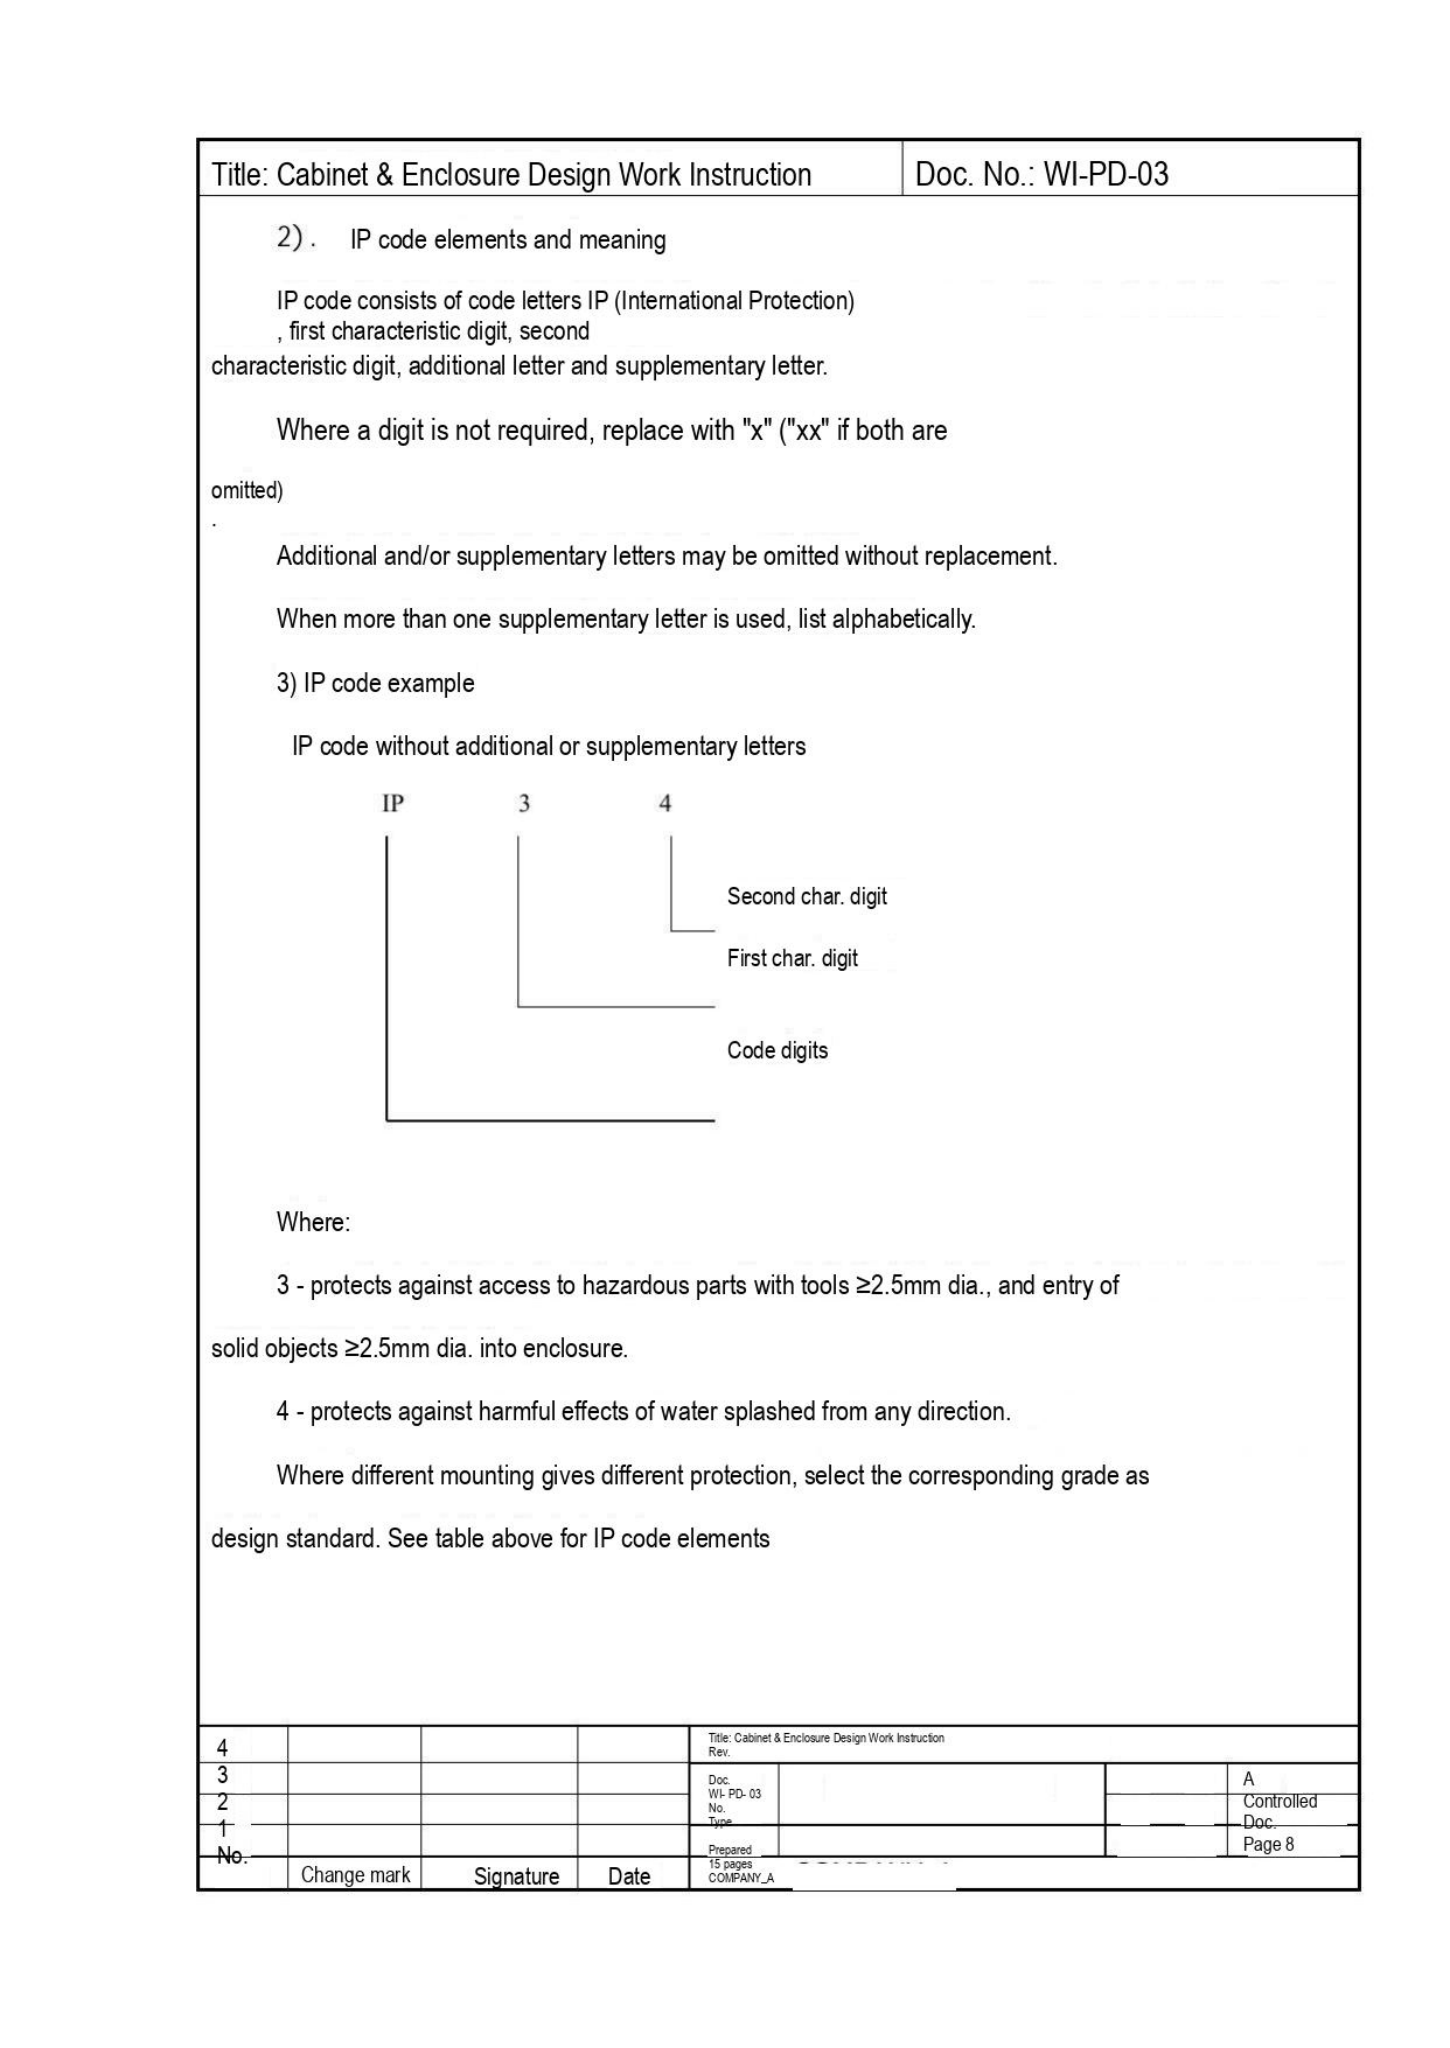| Title: Cabinet & Enclosure Design Work Instruction | Doc. No.: WI-PD-03 |
|---|---|

2）. IP code elements and meaning

IP code consists of code letters IP (International Protection), first characteristic digit, second characteristic digit, additional letter and supplementary letter.

Where a digit is not required, replace with "x" ("xx" if both are omitted).

Additional and/or supplementary letters may be omitted without replacement.

When more than one supplementary letter is used, list alphabetically.

3) IP code example

IP code without additional or supplementary letters

IP 3 4

Second char. digit

First char. digit

Code digits

Where:

3 - protects against access to hazardous parts with tools ≥2.5mm dia., and entry of solid objects ≥2.5mm dia. into enclosure.

4 - protects against harmful effects of water splashed from any direction.

Where different mounting gives different protection, select the corresponding grade as design standard. See table above for IP code elements

| No. | Change mark | Signature | Date |
|---|---|---|---|
| 4 | | | |
| 3 | | | |
| 2 | | | |
| 1 | | | |

Title: Cabinet & Enclosure Design Work Instruction
Rev.
Doc. No. WI- PD- 03
Type
Prepared
15 pages
COMPANY_A
A
Controlled Doc.
Page 8
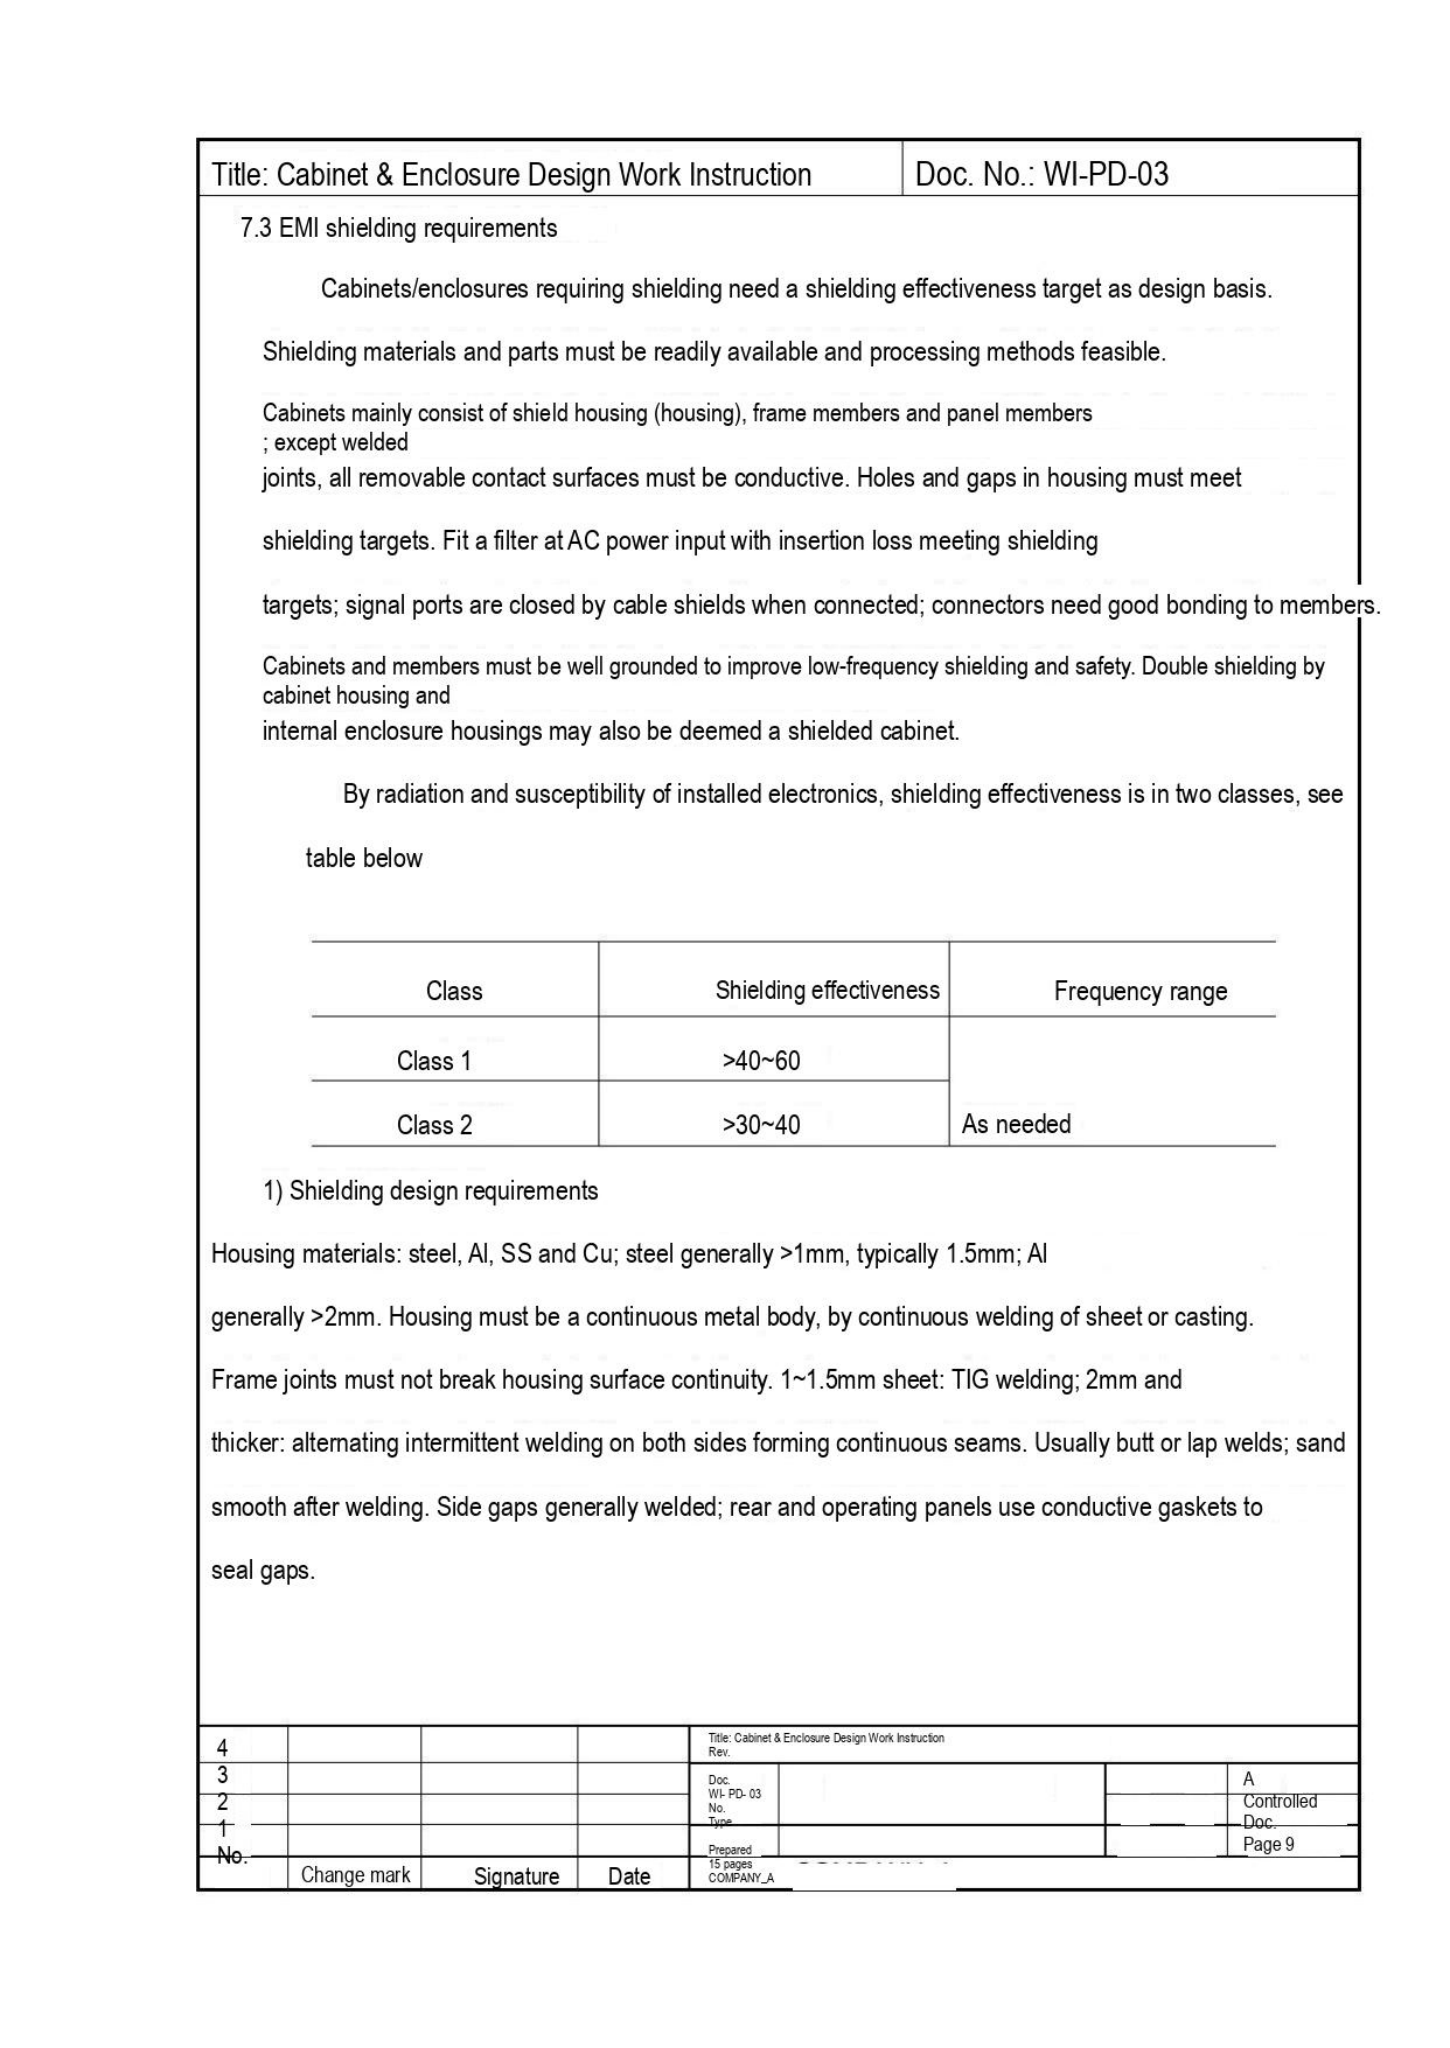Title: Cabinet & Enclosure Design Work Instruction | Doc. No.: WI-PD-03

7.3 EMI shielding requirements

Cabinets/enclosures requiring shielding need a shielding effectiveness target as design basis.

Shielding materials and parts must be readily available and processing methods feasible.

Cabinets mainly consist of shield housing (housing), frame members and panel members ; except welded joints, all removable contact surfaces must be conductive. Holes and gaps in housing must meet shielding targets. Fit a filter at AC power input with insertion loss meeting shielding targets; signal ports are closed by cable shields when connected; connectors need good bonding to members.

Cabinets and members must be well grounded to improve low-frequency shielding and safety. Double shielding by cabinet housing and internal enclosure housings may also be deemed a shielded cabinet.

By radiation and susceptibility of installed electronics, shielding effectiveness is in two classes, see table below

| Class | Shielding effectiveness | Frequency range |
|---|---|---|
| Class 1 | >40~60 | As needed |
| Class 2 | >30~40 | |

1) Shielding design requirements

Housing materials: steel, Al, SS and Cu; steel generally >1mm, typically 1.5mm; Al generally >2mm. Housing must be a continuous metal body, by continuous welding of sheet or casting. Frame joints must not break housing surface continuity. 1~1.5mm sheet: TIG welding; 2mm and thicker: alternating intermittent welding on both sides forming continuous seams. Usually butt or lap welds; sand smooth after welding. Side gaps generally welded; rear and operating panels use conductive gaskets to seal gaps.

| No. | Change mark | Signature | Date |
|---|---|---|---|
| 4 | | | |
| 3 | | | |
| 2 | | | |
| 1 | | | |

Title: Cabinet & Enclosure Design Work Instruction
Rev.
Doc.
WI- PD- 03
No.
Type
Prepared
15 pages
COMPANY_A
A
Controlled
Doc.
Page 9
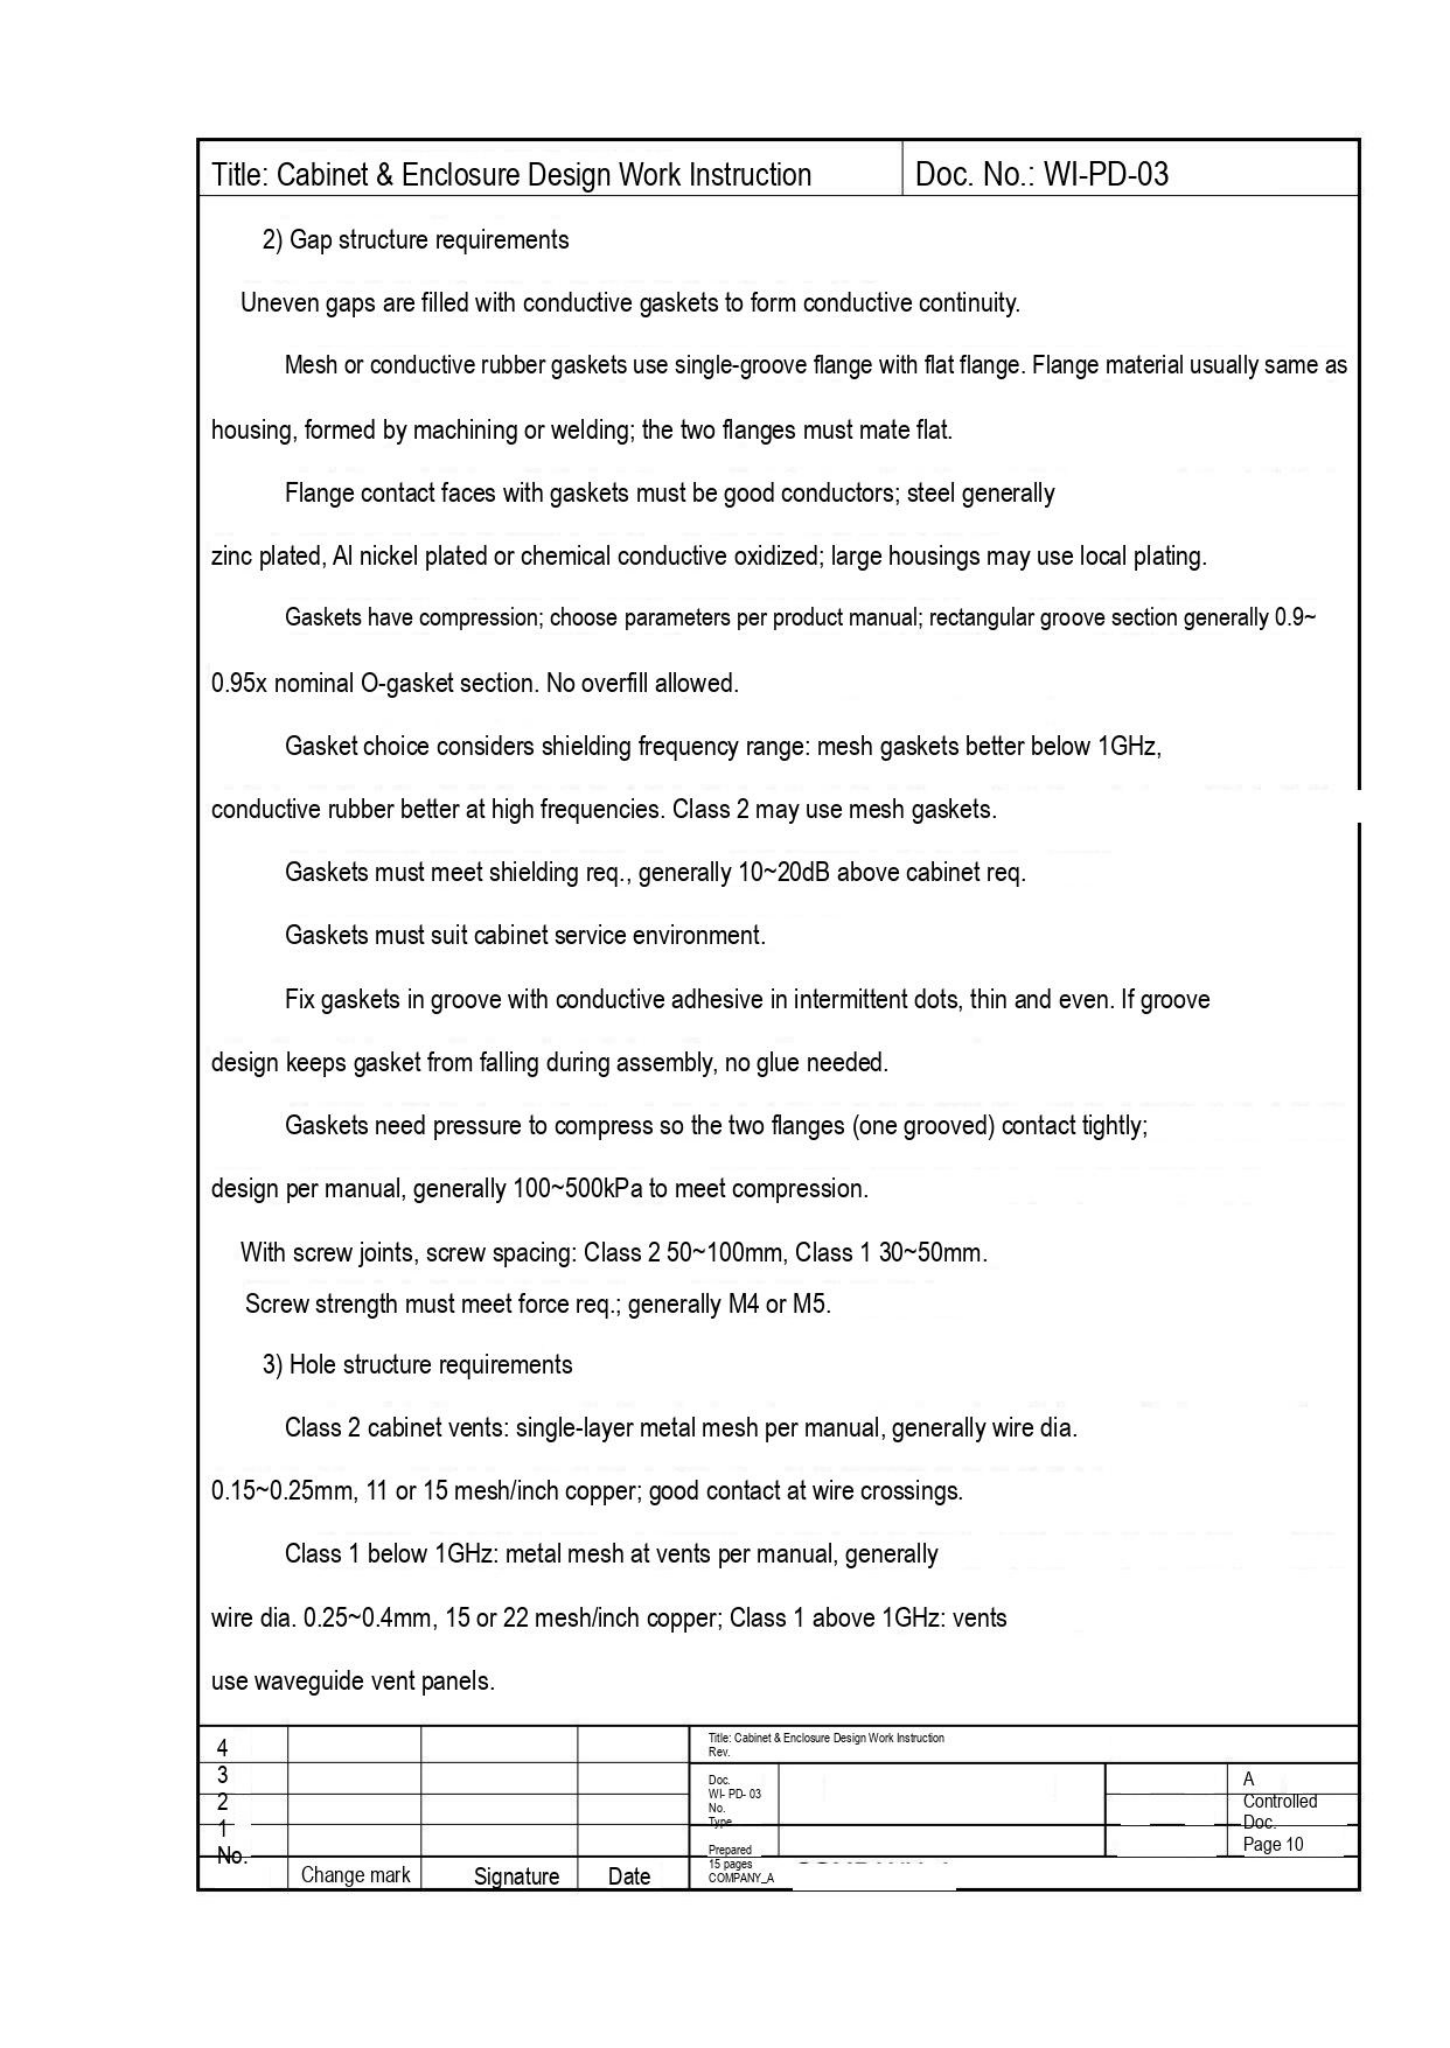| Title: Cabinet & Enclosure Design Work Instruction | Doc. No.: WI-PD-03 |
|---|---|

2) Gap structure requirements

Uneven gaps are filled with conductive gaskets to form conductive continuity.

Mesh or conductive rubber gaskets use single-groove flange with flat flange. Flange material usually same as housing, formed by machining or welding; the two flanges must mate flat.

Flange contact faces with gaskets must be good conductors; steel generally zinc plated, Al nickel plated or chemical conductive oxidized; large housings may use local plating.

Gaskets have compression; choose parameters per product manual; rectangular groove section generally 0.9~0.95x nominal O-gasket section. No overfill allowed.

Gasket choice considers shielding frequency range: mesh gaskets better below 1GHz, conductive rubber better at high frequencies. Class 2 may use mesh gaskets.

Gaskets must meet shielding req., generally 10~20dB above cabinet req.

Gaskets must suit cabinet service environment.

Fix gaskets in groove with conductive adhesive in intermittent dots, thin and even. If groove design keeps gasket from falling during assembly, no glue needed.

Gaskets need pressure to compress so the two flanges (one grooved) contact tightly; design per manual, generally 100~500kPa to meet compression.

With screw joints, screw spacing: Class 2 50~100mm, Class 1 30~50mm.

Screw strength must meet force req.; generally M4 or M5.

3) Hole structure requirements

Class 2 cabinet vents: single-layer metal mesh per manual, generally wire dia. 0.15~0.25mm, 11 or 15 mesh/inch copper; good contact at wire crossings.

Class 1 below 1GHz: metal mesh at vents per manual, generally wire dia. 0.25~0.4mm, 15 or 22 mesh/inch copper; Class 1 above 1GHz: vents use waveguide vent panels.

| 4 | | | | Title: Cabinet & Enclosure Design Work Instruction Rev. | | |
|---|---|---|---|---|---|---|
| 3 | | | | Doc. WI- PD- 03 No. | | A |
| 2 | | | | | | Controlled |
| 1 | | | | Type | | Doc. |
| No. | | | | Prepared | | Page 10 |
| | Change mark | Signature | Date | 15 pages COMPANY_A | | |
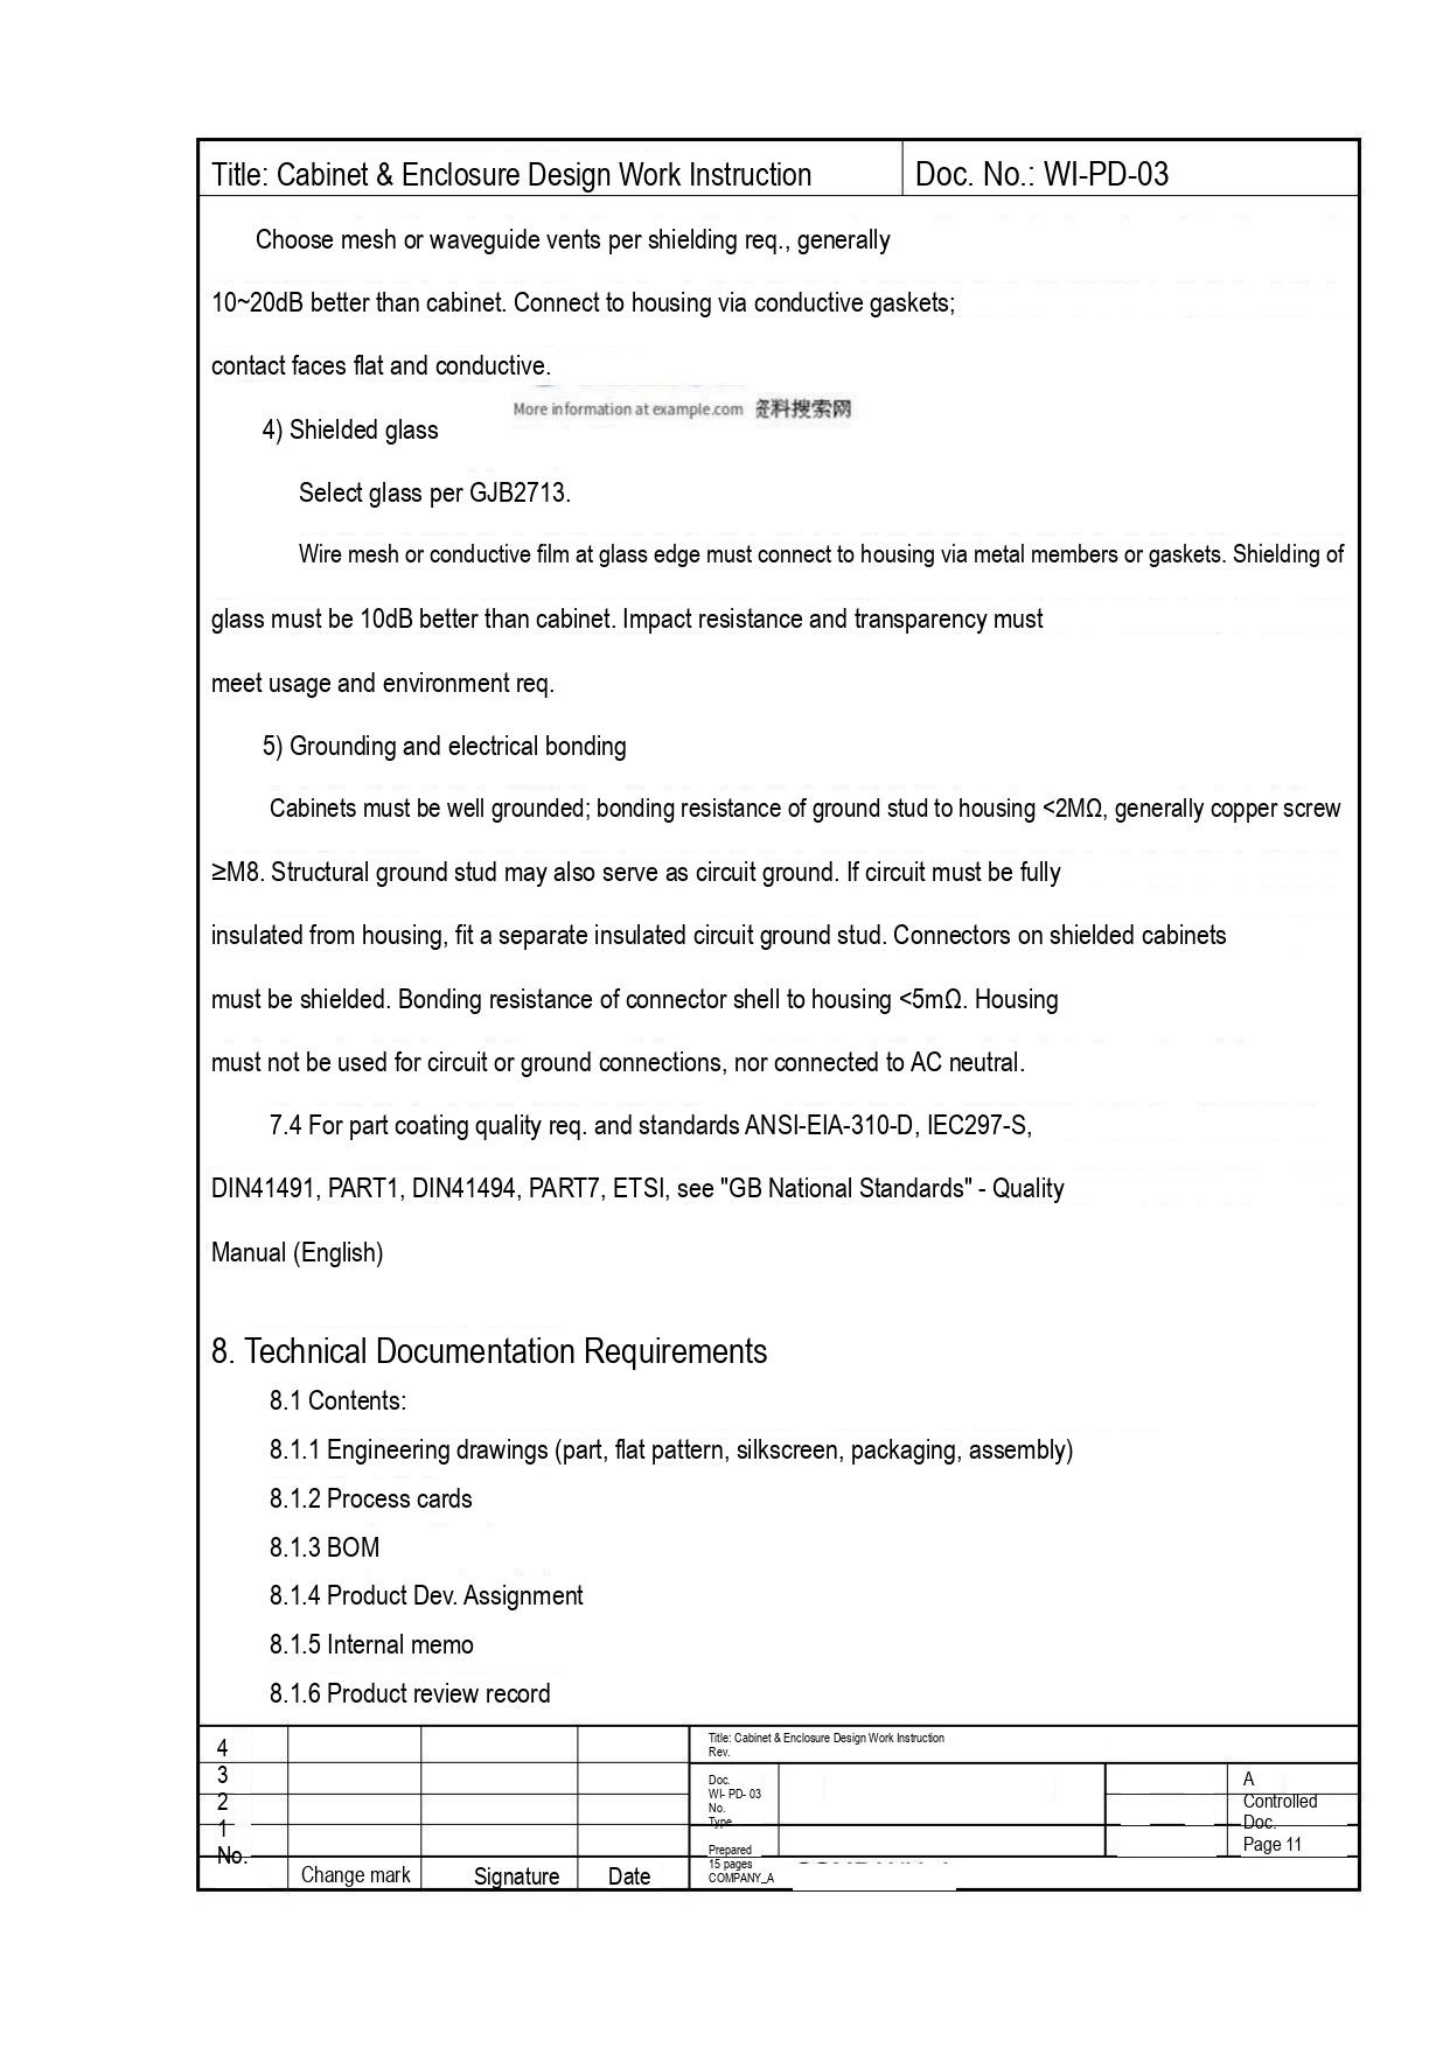| Title: Cabinet & Enclosure Design Work Instruction | Doc. No.: WI-PD-03 |
|---|---|

Choose mesh or waveguide vents per shielding req., generally 10~20dB better than cabinet. Connect to housing via conductive gaskets; contact faces flat and conductive.

More information at example.com 资料搜索网

4) Shielded glass

Select glass per GJB2713.

Wire mesh or conductive film at glass edge must connect to housing via metal members or gaskets. Shielding of glass must be 10dB better than cabinet. Impact resistance and transparency must meet usage and environment req.

5) Grounding and electrical bonding

Cabinets must be well grounded; bonding resistance of ground stud to housing <2MΩ, generally copper screw ≥M8. Structural ground stud may also serve as circuit ground. If circuit must be fully insulated from housing, fit a separate insulated circuit ground stud. Connectors on shielded cabinets must be shielded. Bonding resistance of connector shell to housing <5mΩ. Housing must not be used for circuit or ground connections, nor connected to AC neutral.

7.4 For part coating quality req. and standards ANSI-EIA-310-D, IEC297-S, DIN41491, PART1, DIN41494, PART7, ETSI, see "GB National Standards" - Quality Manual (English)

8. Technical Documentation Requirements

8.1 Contents:

8.1.1 Engineering drawings (part, flat pattern, silkscreen, packaging, assembly)

8.1.2 Process cards

8.1.3 BOM

8.1.4 Product Dev. Assignment

8.1.5 Internal memo

8.1.6 Product review record

| No. | Change mark | Signature | Date | | | |
|---|---|---|---|---|---|---|
| 4 | | | | Title: Cabinet & Enclosure Design Work Instruction Rev. | | |
| 3 | | | | Doc. No. WI- PD- 03 | | A |
| 2 | | | | Type | | Controlled Doc. |
| 1 | | | | Prepared | | Page 11 |
| | | | | 15 pages COMPANY_A | | |
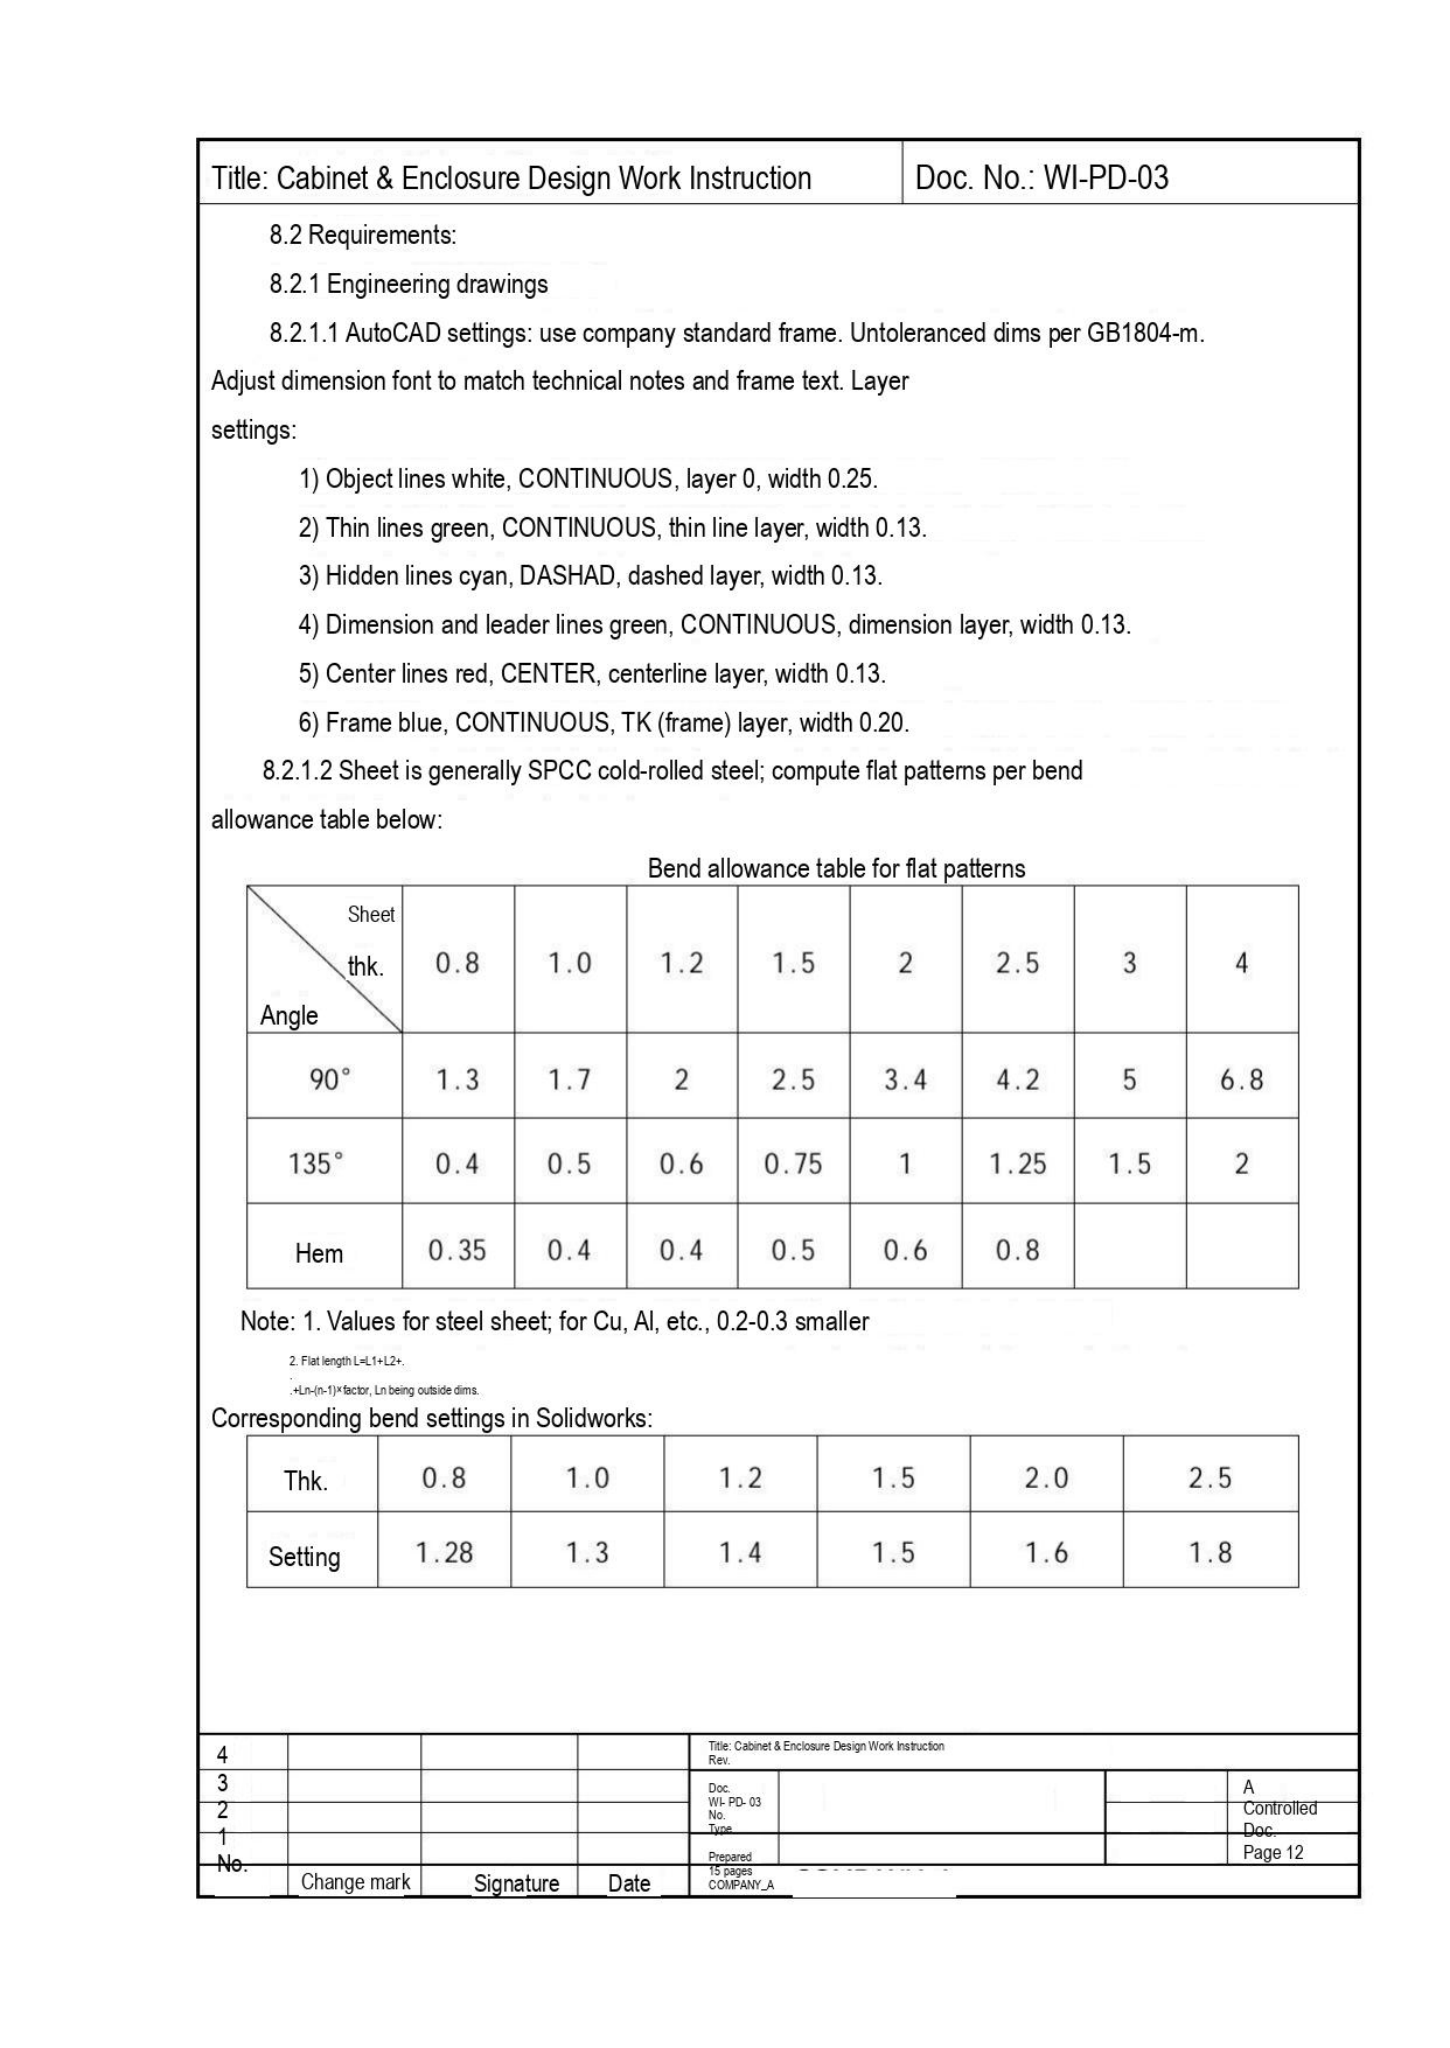Title: Cabinet & Enclosure Design Work Instruction | Doc. No.: WI-PD-03

8.2 Requirements:

8.2.1 Engineering drawings

8.2.1.1 AutoCAD settings: use company standard frame. Untoleranced dims per GB1804-m. Adjust dimension font to match technical notes and frame text. Layer settings:

1) Object lines white, CONTINUOUS, layer 0, width 0.25.

2) Thin lines green, CONTINUOUS, thin line layer, width 0.13.

3) Hidden lines cyan, DASHAD, dashed layer, width 0.13.

4) Dimension and leader lines green, CONTINUOUS, dimension layer, width 0.13.

5) Center lines red, CENTER, centerline layer, width 0.13.

6) Frame blue, CONTINUOUS, TK (frame) layer, width 0.20.

8.2.1.2 Sheet is generally SPCC cold-rolled steel; compute flat patterns per bend allowance table below:

Bend allowance table for flat patterns

| Sheet thk. / Angle | 0.8 | 1.0 | 1.2 | 1.5 | 2 | 2.5 | 3 | 4 |
|---|---|---|---|---|---|---|---|---|
| 90° | 1.3 | 1.7 | 2 | 2.5 | 3.4 | 4.2 | 5 | 6.8 |
| 135° | 0.4 | 0.5 | 0.6 | 0.75 | 1 | 1.25 | 1.5 | 2 |
| Hem | 0.35 | 0.4 | 0.4 | 0.5 | 0.6 | 0.8 | | |

Note: 1. Values for steel sheet; for Cu, Al, etc., 0.2-0.3 smaller

2. Flat length L=L1+L2+.

.+Ln-(n-1)×factor, Ln being outside dims.

Corresponding bend settings in Solidworks:

| Thk. | 0.8 | 1.0 | 1.2 | 1.5 | 2.0 | 2.5 |
|---|---|---|---|---|---|---|
| Setting | 1.28 | 1.3 | 1.4 | 1.5 | 1.6 | 1.8 |

| No. | Change mark | Signature | Date |
|---|---|---|---|
| 4 | | | |
| 3 | | | |
| 2 | | | |
| 1 | | | |

Title: Cabinet & Enclosure Design Work Instruction
Rev.
Doc. No. WI- PD- 03
Type
Prepared
15 pages
COMPANY_A
A Controlled Doc.
Page 12
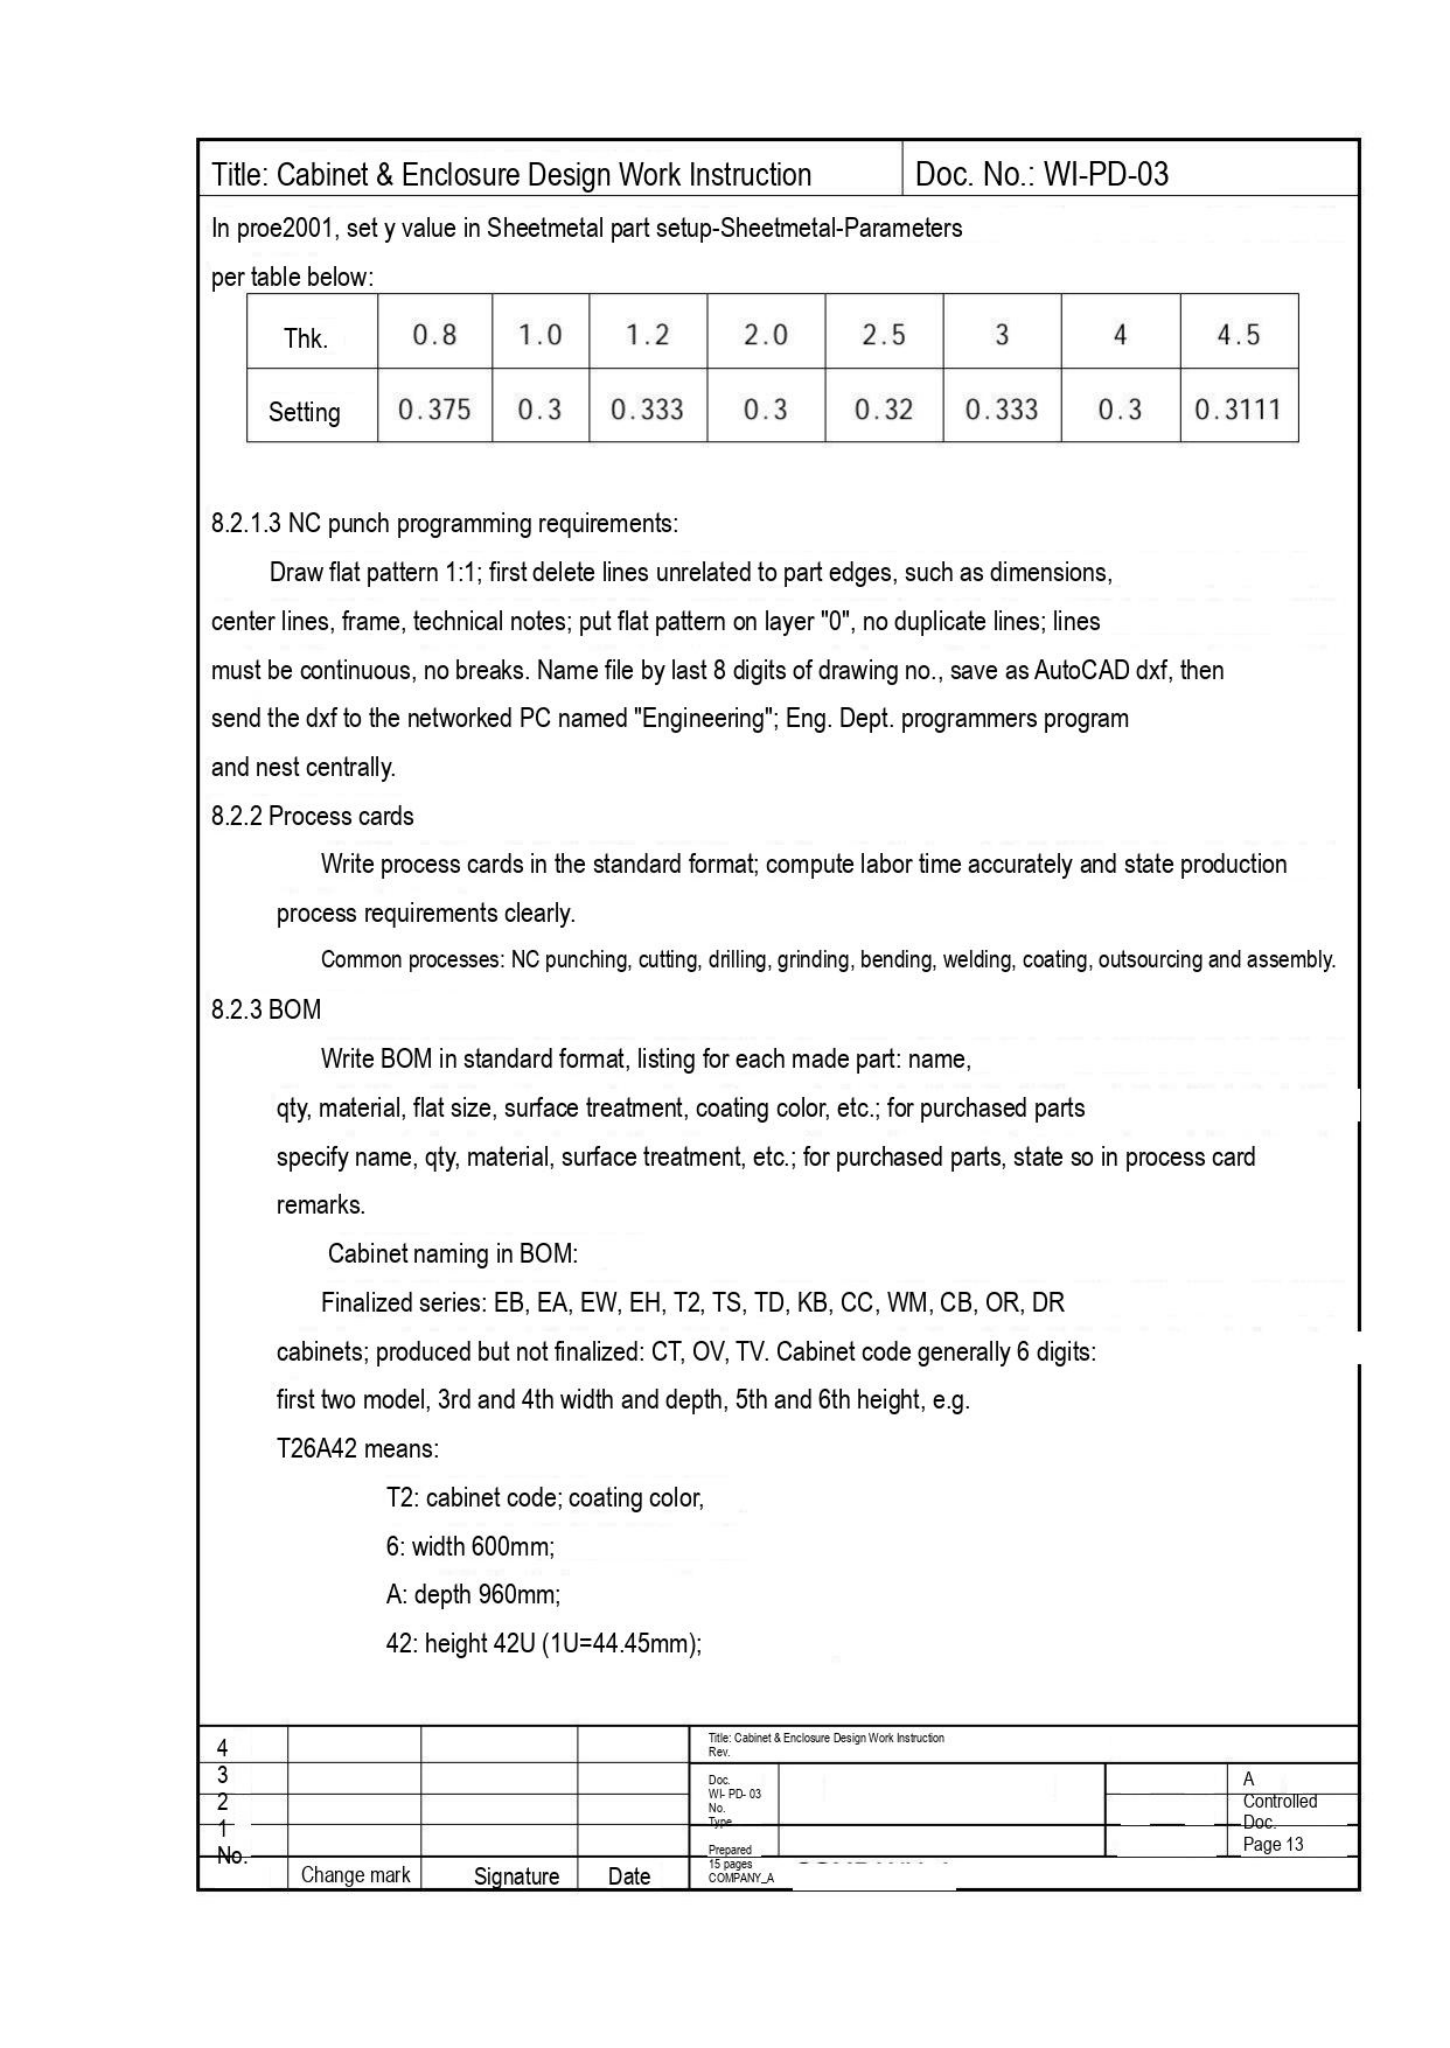Title: Cabinet & Enclosure Design Work Instruction | Doc. No.: WI-PD-03

In proe2001, set y value in Sheetmetal part setup-Sheetmetal-Parameters
per table below:

| Thk. | 0.8 | 1.0 | 1.2 | 2.0 | 2.5 | 3 | 4 | 4.5 |
|---|---|---|---|---|---|---|---|---|
| Setting | 0.375 | 0.3 | 0.333 | 0.3 | 0.32 | 0.333 | 0.3 | 0.3111 |

8.2.1.3 NC punch programming requirements:
Draw flat pattern 1:1; first delete lines unrelated to part edges, such as dimensions, center lines, frame, technical notes; put flat pattern on layer "0", no duplicate lines; lines must be continuous, no breaks. Name file by last 8 digits of drawing no., save as AutoCAD dxf, then send the dxf to the networked PC named "Engineering"; Eng. Dept. programmers program and nest centrally.

8.2.2 Process cards
Write process cards in the standard format; compute labor time accurately and state production process requirements clearly.
Common processes: NC punching, cutting, drilling, grinding, bending, welding, coating, outsourcing and assembly.

8.2.3 BOM
Write BOM in standard format, listing for each made part: name, qty, material, flat size, surface treatment, coating color, etc.; for purchased parts specify name, qty, material, surface treatment, etc.; for purchased parts, state so in process card remarks.
Cabinet naming in BOM:
Finalized series: EB, EA, EW, EH, T2, TS, TD, KB, CC, WM, CB, OR, DR cabinets; produced but not finalized: CT, OV, TV. Cabinet code generally 6 digits: first two model, 3rd and 4th width and depth, 5th and 6th height, e.g.
T26A42 means:
T2: cabinet code; coating color,
6: width 600mm;
A: depth 960mm;
42: height 42U (1U=44.45mm);

| | | | | Title: Cabinet & Enclosure Design Work Instruction<br>Rev. | | |
|---|---|---|---|---|---|---|
| 4 | | | | Doc.<br>WI- PD- 03<br>No.<br>Type | | A<br>Controlled<br>Doc. |
| 3 | | | | | | |
| 2 | | | | | | |
| 1 | | | | Prepared | | Page 13 |
| No. | Change mark | Signature | Date | 15 pages<br>COMPANY_A | | |